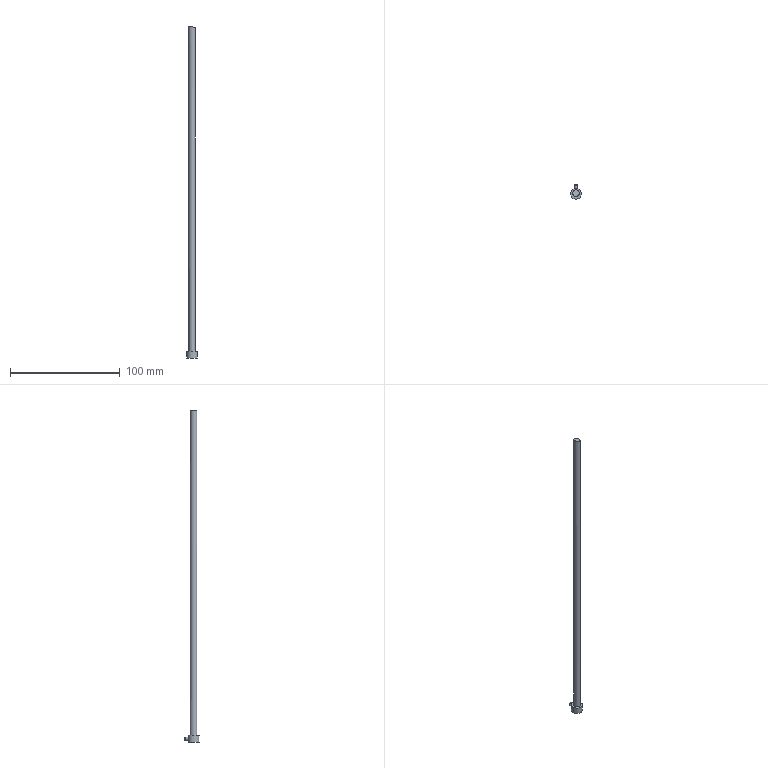Part | STEP file | E106-17-310 | 1 solid | 8 faces | box 10 x 13 x 302.496 mm | volume 8853 mm3 | cylinder 3 | plane 3 | spline 1 | cone 1 | commonest cylinder face diameters 3 x1 6 x1 10 x1